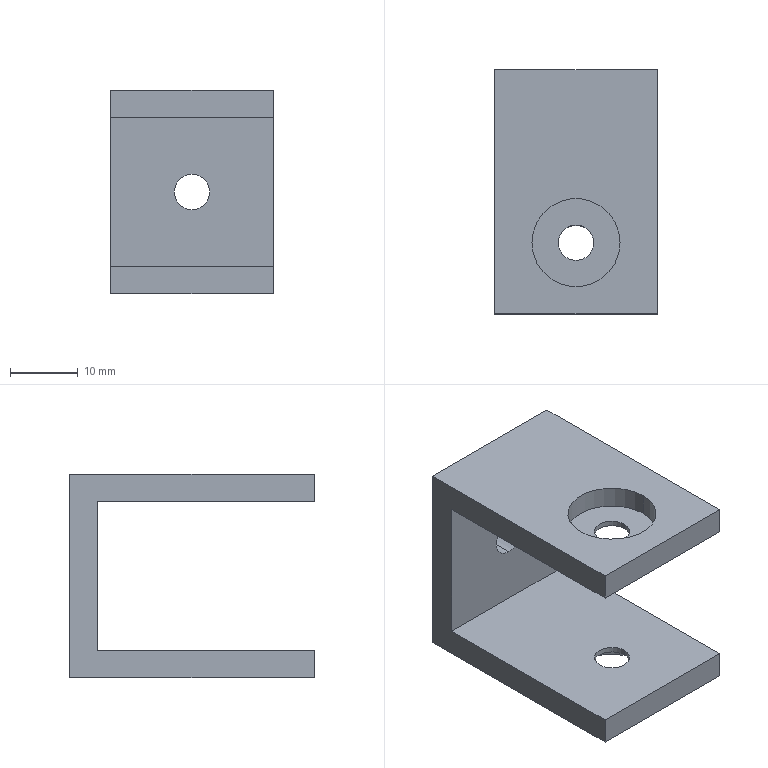Part | SolidWorks | features ICE 12, Extrusion 1, MirrorPattern 1 | 1 solid | 22 faces | box 23.897 x 36 x 30 mm | volume 8017 mm3 | plane 12 | cylinder 10 | commonest cylinder face diameters 5.2 x6 13 x4
STEP:
#1=CARTESIAN_POINT('',(6.5,-14.25,26.8));
#2=VERTEX_POINT('',#1);
#3=CARTESIAN_POINT('',(-6.5,-14.25,26.8));
#4=VERTEX_POINT('',#3);
#5=CARTESIAN_POINT('',(0.,-14.25,26.8));
#6=DIRECTION('',(0.,0.,-1.));
#7=DIRECTION('',(-1.,0.,0.));
#8=AXIS2_PLACEMENT_3D('',#5,#6,#7);
#9=CIRCLE('',#8,6.5);
#10=EDGE_CURVE('',#2,#4,#9,.T.);
#11=ORIENTED_EDGE('',*,*,#10,.T.);
#12=CARTESIAN_POINT('',(-6.5,-14.25,30.));
#13=VERTEX_POINT('',#12);
#14=CARTESIAN_POINT('',(-6.5,-14.25,26.8));
#15=DIRECTION('',(0.,0.,1.));
#16=VECTOR('',#15,1000.);
#17=LINE('',#14,#16);
#18=EDGE_CURVE('',#4,#13,#17,.T.);
#19=ORIENTED_EDGE('',*,*,#18,.T.);
#20=CARTESIAN_POINT('',(6.5,-14.25,30.));
#21=VERTEX_POINT('',#20);
#22=CARTESIAN_POINT('',(0.,-14.25,30.));
#23=DIRECTION('',(0.,0.,-1.));
#24=DIRECTION('',(-1.,0.,0.));
#25=AXIS2_PLACEMENT_3D('',#22,#23,#24);
#26=CIRCLE('',#25,6.5);
#27=EDGE_CURVE('',#21,#13,#26,.T.);
#28=ORIENTED_EDGE('',*,*,#27,.F.);
#29=CARTESIAN_POINT('',(6.5,-14.25,26.8));
#30=DIRECTION('',(0.,0.,1.));
#31=VECTOR('',#30,1000.);
#32=LINE('',#29,#31);
#33=EDGE_CURVE('',#2,#21,#32,.T.);
#34=ORIENTED_EDGE('',*,*,#33,.F.);
#35=EDGE_LOOP('',(#11,#19,#28,#34));
#36=FACE_OUTER_BOUND('',#35,.T.);
#37=CARTESIAN_POINT('',(0.,-14.25,26.8));
#38=DIRECTION('',(0.,0.,1.));
#39=DIRECTION('',(1.,0.,0.));
#40=AXIS2_PLACEMENT_3D('',#37,#38,#39);
#41=CYLINDRICAL_SURFACE('',#40,6.5);
#42=ADVANCED_FACE('',(#36),#41,.F.);
#43=CARTESIAN_POINT('',(6.5,-14.25,3.2));
#44=VERTEX_POINT('',#43);
#45=CARTESIAN_POINT('',(-6.5,-14.25,3.2));
#46=VERTEX_POINT('',#45);
#47=CARTESIAN_POINT('',(0.,-14.25,3.2));
#48=DIRECTION('',(0.,0.,-1.));
#49=DIRECTION('',(-1.,0.,0.));
#50=AXIS2_PLACEMENT_3D('',#47,#48,#49);
#51=CIRCLE('',#50,6.5);
#52=EDGE_CURVE('',#44,#46,#51,.T.);
#53=ORIENTED_EDGE('',*,*,#52,.F.);
#54=CARTESIAN_POINT('',(6.5,-14.25,0.));
#55=VERTEX_POINT('',#54);
#56=CARTESIAN_POINT('',(6.5,-14.25,3.2));
#57=DIRECTION('',(0.,0.,-1.));
#58=VECTOR('',#57,1000.);
#59=LINE('',#56,#58);
#60=EDGE_CURVE('',#44,#55,#59,.T.);
#61=ORIENTED_EDGE('',*,*,#60,.T.);
#62=CARTESIAN_POINT('',(-6.5,-14.25,0.));
#63=VERTEX_POINT('',#62);
#64=CARTESIAN_POINT('',(0.,-14.25,0.));
#65=DIRECTION('',(0.,0.,-1.));
#66=DIRECTION('',(-1.,0.,0.));
#67=AXIS2_PLACEMENT_3D('',#64,#65,#66);
#68=CIRCLE('',#67,6.5);
#69=EDGE_CURVE('',#55,#63,#68,.T.);
#70=ORIENTED_EDGE('',*,*,#69,.T.);
#71=CARTESIAN_POINT('',(-6.5,-14.25,3.2));
#72=DIRECTION('',(0.,0.,-1.));
#73=VECTOR('',#72,1000.);
#74=LINE('',#71,#73);
#75=EDGE_CURVE('',#46,#63,#74,.T.);
#76=ORIENTED_EDGE('',*,*,#75,.F.);
#77=EDGE_LOOP('',(#53,#61,#70,#76));
#78=FACE_OUTER_BOUND('',#77,.T.);
#79=CARTESIAN_POINT('',(0.,-14.25,3.2));
#80=DIRECTION('',(0.,0.,-1.));
#81=DIRECTION('',(-1.,0.,0.));
#82=AXIS2_PLACEMENT_3D('',#79,#80,#81);
#83=CYLINDRICAL_SURFACE('',#82,6.5);
#84=ADVANCED_FACE('',(#78),#83,.F.);
#85=CARTESIAN_POINT('',(0.,7.25,12.4));
#86=VERTEX_POINT('',#85);
#87=CARTESIAN_POINT('',(0.,7.25,17.6));
#88=VERTEX_POINT('',#87);
#89=CARTESIAN_POINT('',(0.,7.25,15.));
#90=DIRECTION('',(0.,1.,0.));
#91=DIRECTION('',(0.,0.,1.));
#92=AXIS2_PLACEMENT_3D('',#89,#90,#91);
#93=CIRCLE('',#92,2.6);
#94=EDGE_CURVE('',#86,#88,#93,.T.);
#95=ORIENTED_EDGE('',*,*,#94,.F.);
#96=CARTESIAN_POINT('',(0.,11.25,12.4));
#97=VERTEX_POINT('',#96);
#98=CARTESIAN_POINT('',(0.,-19.75,12.4));
#99=DIRECTION('',(0.,1.,0.));
#100=VECTOR('',#99,1000.);
#101=LINE('',#98,#100);
#102=EDGE_CURVE('',#86,#97,#101,.T.);
#103=ORIENTED_EDGE('',*,*,#102,.T.);
#104=CARTESIAN_POINT('',(0.,11.25,17.6));
#105=VERTEX_POINT('',#104);
#106=CARTESIAN_POINT('',(0.,11.25,15.));
#107=DIRECTION('',(0.,1.,0.));
#108=DIRECTION('',(0.,0.,1.));
#109=AXIS2_PLACEMENT_3D('',#106,#107,#108);
#110=CIRCLE('',#109,2.6);
#111=EDGE_CURVE('',#97,#105,#110,.T.);
#112=ORIENTED_EDGE('',*,*,#111,.T.);
#113=CARTESIAN_POINT('',(0.,-19.75,17.6));
#114=DIRECTION('',(0.,1.,0.));
#115=VECTOR('',#114,1000.);
#116=LINE('',#113,#115);
#117=EDGE_CURVE('',#88,#105,#116,.T.);
#118=ORIENTED_EDGE('',*,*,#117,.F.);
#119=EDGE_LOOP('',(#95,#103,#112,#118));
#120=FACE_OUTER_BOUND('',#119,.T.);
#121=CARTESIAN_POINT('',(0.,-19.75,15.));
#122=DIRECTION('',(0.,1.,0.));
#123=DIRECTION('',(0.,0.,1.));
#124=AXIS2_PLACEMENT_3D('',#121,#122,#123);
#125=CYLINDRICAL_SURFACE('',#124,2.6);
#126=ADVANCED_FACE('',(#120),#125,.F.);
#127=CARTESIAN_POINT('',(-2.6,-14.25,3.2));
#128=VERTEX_POINT('',#127);
#129=CARTESIAN_POINT('',(2.6,-14.25,3.2));
#130=VERTEX_POINT('',#129);
#131=CARTESIAN_POINT('',(0.,-14.25,3.2));
#132=DIRECTION('',(0.,0.,1.));
#133=DIRECTION('',(-1.,0.,0.));
#134=AXIS2_PLACEMENT_3D('',#131,#132,#133);
#135=CIRCLE('',#134,2.6);
#136=EDGE_CURVE('',#128,#130,#135,.T.);
#137=ORIENTED_EDGE('',*,*,#136,.F.);
#138=CARTESIAN_POINT('',(-2.6,-14.25,4.));
#139=VERTEX_POINT('',#138);
#140=CARTESIAN_POINT('',(-2.6,-14.25,0.));
#141=DIRECTION('',(0.,0.,1.));
#142=VECTOR('',#141,1000.);
#143=LINE('',#140,#142);
#144=EDGE_CURVE('',#128,#139,#143,.T.);
#145=ORIENTED_EDGE('',*,*,#144,.T.);
#146=CARTESIAN_POINT('',(2.6,-14.25,4.));
#147=VERTEX_POINT('',#146);
#148=CARTESIAN_POINT('',(0.,-14.25,4.));
#149=DIRECTION('',(0.,0.,-1.));
#150=DIRECTION('',(0.,1.,0.));
#151=AXIS2_PLACEMENT_3D('',#148,#149,#150);
#152=CIRCLE('',#151,2.6);
#153=EDGE_CURVE('',#147,#139,#152,.T.);
#154=ORIENTED_EDGE('',*,*,#153,.F.);
#155=CARTESIAN_POINT('',(2.6,-14.25,0.));
#156=DIRECTION('',(0.,0.,1.));
#157=VECTOR('',#156,1000.);
#158=LINE('',#155,#157);
#159=EDGE_CURVE('',#130,#147,#158,.T.);
#160=ORIENTED_EDGE('',*,*,#159,.F.);
#161=EDGE_LOOP('',(#137,#145,#154,#160));
#162=FACE_OUTER_BOUND('',#161,.T.);
#163=CARTESIAN_POINT('',(0.,-14.25,0.));
#164=DIRECTION('',(0.,0.,1.));
#165=DIRECTION('',(1.,0.,0.));
#166=AXIS2_PLACEMENT_3D('',#163,#164,#165);
#167=CYLINDRICAL_SURFACE('',#166,2.6);
#168=ADVANCED_FACE('',(#162),#167,.F.);
#169=CARTESIAN_POINT('',(-2.6,-14.25,26.));
#170=VERTEX_POINT('',#169);
#171=CARTESIAN_POINT('',(2.6,-14.25,26.));
#172=VERTEX_POINT('',#171);
#173=CARTESIAN_POINT('',(0.,-14.25,26.));
#174=DIRECTION('',(0.,0.,1.));
#175=DIRECTION('',(0.,-1.,0.));
#176=AXIS2_PLACEMENT_3D('',#173,#174,#175);
#177=CIRCLE('',#176,2.6);
#178=EDGE_CURVE('',#170,#172,#177,.T.);
#179=ORIENTED_EDGE('',*,*,#178,.F.);
#180=CARTESIAN_POINT('',(-2.6,-14.25,26.8));
#181=VERTEX_POINT('',#180);
#182=CARTESIAN_POINT('',(-2.6,-14.25,0.));
#183=DIRECTION('',(0.,0.,1.));
#184=VECTOR('',#183,1000.);
#185=LINE('',#182,#184);
#186=EDGE_CURVE('',#170,#181,#185,.T.);
#187=ORIENTED_EDGE('',*,*,#186,.T.);
#188=CARTESIAN_POINT('',(2.6,-14.25,26.8));
#189=VERTEX_POINT('',#188);
#190=CARTESIAN_POINT('',(0.,-14.25,26.8));
#191=DIRECTION('',(0.,0.,-1.));
#192=DIRECTION('',(1.,0.,0.));
#193=AXIS2_PLACEMENT_3D('',#190,#191,#192);
#194=CIRCLE('',#193,2.6);
#195=EDGE_CURVE('',#189,#181,#194,.T.);
#196=ORIENTED_EDGE('',*,*,#195,.F.);
#197=CARTESIAN_POINT('',(2.6,-14.25,0.));
#198=DIRECTION('',(0.,0.,1.));
#199=VECTOR('',#198,1000.);
#200=LINE('',#197,#199);
#201=EDGE_CURVE('',#172,#189,#200,.T.);
#202=ORIENTED_EDGE('',*,*,#201,.F.);
#203=EDGE_LOOP('',(#179,#187,#196,#202));
#204=FACE_OUTER_BOUND('',#203,.T.);
#205=CARTESIAN_POINT('',(0.,-14.25,0.));
#206=DIRECTION('',(0.,0.,1.));
#207=DIRECTION('',(1.,0.,0.));
#208=AXIS2_PLACEMENT_3D('',#205,#206,#207);
#209=CYLINDRICAL_SURFACE('',#208,2.6);
#210=ADVANCED_FACE('',(#204),#209,.F.);
#211=ORIENTED_EDGE('',*,*,#186,.F.);
#212=CARTESIAN_POINT('',(0.,-14.25,26.));
#213=DIRECTION('',(0.,0.,1.));
#214=DIRECTION('',(0.,-1.,0.));
#215=AXIS2_PLACEMENT_3D('',#212,#213,#214);
#216=CIRCLE('',#215,2.6);
#217=EDGE_CURVE('',#172,#170,#216,.T.);
#218=ORIENTED_EDGE('',*,*,#217,.F.);
#219=ORIENTED_EDGE('',*,*,#201,.T.);
#220=CARTESIAN_POINT('',(0.,-14.25,26.8));
#221=DIRECTION('',(0.,0.,-1.));
#222=DIRECTION('',(1.,0.,0.));
#223=AXIS2_PLACEMENT_3D('',#220,#221,#222);
#224=CIRCLE('',#223,2.6);
#225=EDGE_CURVE('',#181,#189,#224,.T.);
#226=ORIENTED_EDGE('',*,*,#225,.F.);
#227=EDGE_LOOP('',(#211,#218,#219,#226));
#228=FACE_OUTER_BOUND('',#227,.T.);
#229=CARTESIAN_POINT('',(0.,-14.25,0.));
#230=DIRECTION('',(0.,0.,1.));
#231=DIRECTION('',(1.,0.,0.));
#232=AXIS2_PLACEMENT_3D('',#229,#230,#231);
#233=CYLINDRICAL_SURFACE('',#232,2.6);
#234=ADVANCED_FACE('',(#228),#233,.F.);
#235=ORIENTED_EDGE('',*,*,#144,.F.);
#236=CARTESIAN_POINT('',(0.,-14.25,3.2));
#237=DIRECTION('',(0.,0.,1.));
#238=DIRECTION('',(-1.,0.,0.));
#239=AXIS2_PLACEMENT_3D('',#236,#237,#238);
#240=CIRCLE('',#239,2.6);
#241=EDGE_CURVE('',#130,#128,#240,.T.);
#242=ORIENTED_EDGE('',*,*,#241,.F.);
#243=ORIENTED_EDGE('',*,*,#159,.T.);
#244=CARTESIAN_POINT('',(0.,-14.25,4.));
#245=DIRECTION('',(0.,0.,-1.));
#246=DIRECTION('',(0.,1.,0.));
#247=AXIS2_PLACEMENT_3D('',#244,#245,#246);
#248=CIRCLE('',#247,2.6);
#249=EDGE_CURVE('',#139,#147,#248,.T.);
#250=ORIENTED_EDGE('',*,*,#249,.F.);
#251=EDGE_LOOP('',(#235,#242,#243,#250));
#252=FACE_OUTER_BOUND('',#251,.T.);
#253=CARTESIAN_POINT('',(0.,-14.25,0.));
#254=DIRECTION('',(0.,0.,1.));
#255=DIRECTION('',(1.,0.,0.));
#256=AXIS2_PLACEMENT_3D('',#253,#254,#255);
#257=CYLINDRICAL_SURFACE('',#256,2.6);
#258=ADVANCED_FACE('',(#252),#257,.F.);
#259=CARTESIAN_POINT('',(11.948,-24.75,0.));
#260=VERTEX_POINT('',#259);
#261=CARTESIAN_POINT('',(11.948,11.25,0.));
#262=VERTEX_POINT('',#261);
#263=CARTESIAN_POINT('',(11.948,12.75,0.));
#264=DIRECTION('',(0.,1.,0.));
#265=VECTOR('',#264,1000.);
#266=LINE('',#263,#265);
#267=EDGE_CURVE('',#260,#262,#266,.T.);
#268=ORIENTED_EDGE('',*,*,#267,.T.);
#269=CARTESIAN_POINT('',(11.948,11.25,30.));
#270=VERTEX_POINT('',#269);
#271=CARTESIAN_POINT('',(11.948,11.25,30.));
#272=DIRECTION('',(0.,0.,-1.));
#273=VECTOR('',#272,1000.);
#274=LINE('',#271,#273);
#275=EDGE_CURVE('',#270,#262,#274,.T.);
#276=ORIENTED_EDGE('',*,*,#275,.F.);
#277=CARTESIAN_POINT('',(11.948,-24.75,30.));
#278=VERTEX_POINT('',#277);
#279=CARTESIAN_POINT('',(11.948,12.75,30.));
#280=DIRECTION('',(0.,1.,0.));
#281=VECTOR('',#280,1000.);
#282=LINE('',#279,#281);
#283=EDGE_CURVE('',#278,#270,#282,.T.);
#284=ORIENTED_EDGE('',*,*,#283,.F.);
#285=CARTESIAN_POINT('',(11.948,-24.75,26.));
#286=VERTEX_POINT('',#285);
#287=CARTESIAN_POINT('',(11.948,-24.75,26.));
#288=DIRECTION('',(0.,0.,1.));
#289=VECTOR('',#288,1000.);
#290=LINE('',#287,#289);
#291=EDGE_CURVE('',#286,#278,#290,.T.);
#292=ORIENTED_EDGE('',*,*,#291,.F.);
#293=CARTESIAN_POINT('',(11.948,7.25,26.));
#294=VERTEX_POINT('',#293);
#295=CARTESIAN_POINT('',(11.948,7.25,26.));
#296=DIRECTION('',(0.,-1.,0.));
#297=VECTOR('',#296,1000.);
#298=LINE('',#295,#297);
#299=EDGE_CURVE('',#294,#286,#298,.T.);
#300=ORIENTED_EDGE('',*,*,#299,.F.);
#301=CARTESIAN_POINT('',(11.948,7.25,4.));
#302=VERTEX_POINT('',#301);
#303=CARTESIAN_POINT('',(11.948,7.25,20.));
#304=DIRECTION('',(0.,0.,1.));
#305=VECTOR('',#304,1000.);
#306=LINE('',#303,#305);
#307=EDGE_CURVE('',#302,#294,#306,.T.);
#308=ORIENTED_EDGE('',*,*,#307,.F.);
#309=CARTESIAN_POINT('',(11.948,-24.75,4.));
#310=VERTEX_POINT('',#309);
#311=CARTESIAN_POINT('',(11.948,7.25,4.));
#312=DIRECTION('',(0.,1.,0.));
#313=VECTOR('',#312,1000.);
#314=LINE('',#311,#313);
#315=EDGE_CURVE('',#310,#302,#314,.T.);
#316=ORIENTED_EDGE('',*,*,#315,.F.);
#317=CARTESIAN_POINT('',(11.948,-24.75,0.));
#318=DIRECTION('',(0.,0.,1.));
#319=VECTOR('',#318,1000.);
#320=LINE('',#317,#319);
#321=EDGE_CURVE('',#260,#310,#320,.T.);
#322=ORIENTED_EDGE('',*,*,#321,.F.);
#323=EDGE_LOOP('',(#268,#276,#284,#292,#300,#308,#316,#322));
#324=FACE_OUTER_BOUND('',#323,.T.);
#325=CARTESIAN_POINT('',(11.948,12.75,30.));
#326=DIRECTION('',(-1.,0.,0.));
#327=DIRECTION('',(0.,0.,1.));
#328=AXIS2_PLACEMENT_3D('',#325,#326,#327);
#329=PLANE('',#328);
#330=ADVANCED_FACE('',(#324),#329,.F.);
#331=CARTESIAN_POINT('',(-11.948,11.25,30.));
#332=VERTEX_POINT('',#331);
#333=CARTESIAN_POINT('',(-11.948,-24.75,30.));
#334=VERTEX_POINT('',#333);
#335=CARTESIAN_POINT('',(-11.948,12.75,30.));
#336=DIRECTION('',(0.,-1.,0.));
#337=VECTOR('',#336,1000.);
#338=LINE('',#335,#337);
#339=EDGE_CURVE('',#332,#334,#338,.T.);
#340=ORIENTED_EDGE('',*,*,#339,.F.);
#341=CARTESIAN_POINT('',(-11.948,11.25,0.));
#342=VERTEX_POINT('',#341);
#343=CARTESIAN_POINT('',(-11.948,11.25,30.));
#344=DIRECTION('',(0.,0.,-1.));
#345=VECTOR('',#344,1000.);
#346=LINE('',#343,#345);
#347=EDGE_CURVE('',#332,#342,#346,.T.);
#348=ORIENTED_EDGE('',*,*,#347,.T.);
#349=CARTESIAN_POINT('',(-11.948,-24.75,0.));
#350=VERTEX_POINT('',#349);
#351=CARTESIAN_POINT('',(-11.948,12.75,0.));
#352=DIRECTION('',(0.,-1.,0.));
#353=VECTOR('',#352,1000.);
#354=LINE('',#351,#353);
#355=EDGE_CURVE('',#342,#350,#354,.T.);
#356=ORIENTED_EDGE('',*,*,#355,.T.);
#357=CARTESIAN_POINT('',(-11.948,-24.75,4.));
#358=VERTEX_POINT('',#357);
#359=CARTESIAN_POINT('',(-11.948,-24.75,4.));
#360=DIRECTION('',(0.,0.,-1.));
#361=VECTOR('',#360,1000.);
#362=LINE('',#359,#361);
#363=EDGE_CURVE('',#358,#350,#362,.T.);
#364=ORIENTED_EDGE('',*,*,#363,.F.);
#365=CARTESIAN_POINT('',(-11.948,7.25,4.));
#366=VERTEX_POINT('',#365);
#367=CARTESIAN_POINT('',(-11.948,7.25,4.));
#368=DIRECTION('',(0.,-1.,0.));
#369=VECTOR('',#368,1000.);
#370=LINE('',#367,#369);
#371=EDGE_CURVE('',#366,#358,#370,.T.);
#372=ORIENTED_EDGE('',*,*,#371,.F.);
#373=CARTESIAN_POINT('',(-11.948,7.25,26.));
#374=VERTEX_POINT('',#373);
#375=CARTESIAN_POINT('',(-11.948,7.25,20.));
#376=DIRECTION('',(0.,0.,1.));
#377=VECTOR('',#376,1000.);
#378=LINE('',#375,#377);
#379=EDGE_CURVE('',#366,#374,#378,.T.);
#380=ORIENTED_EDGE('',*,*,#379,.T.);
#381=CARTESIAN_POINT('',(-11.948,-24.75,26.));
#382=VERTEX_POINT('',#381);
#383=CARTESIAN_POINT('',(-11.948,7.25,26.));
#384=DIRECTION('',(0.,1.,0.));
#385=VECTOR('',#384,1000.);
#386=LINE('',#383,#385);
#387=EDGE_CURVE('',#382,#374,#386,.T.);
#388=ORIENTED_EDGE('',*,*,#387,.F.);
#389=CARTESIAN_POINT('',(-11.948,-24.75,30.));
#390=DIRECTION('',(0.,0.,-1.));
#391=VECTOR('',#390,1000.);
#392=LINE('',#389,#391);
#393=EDGE_CURVE('',#334,#382,#392,.T.);
#394=ORIENTED_EDGE('',*,*,#393,.F.);
#395=EDGE_LOOP('',(#340,#348,#356,#364,#372,#380,#388,#394));
#396=FACE_OUTER_BOUND('',#395,.T.);
#397=CARTESIAN_POINT('',(-11.948,12.75,30.));
#398=DIRECTION('',(1.,0.,0.));
#399=DIRECTION('',(0.,0.,-1.));
#400=AXIS2_PLACEMENT_3D('',#397,#398,#399);
#401=PLANE('',#400);
#402=ADVANCED_FACE('',(#396),#401,.F.);
#403=ORIENTED_EDGE('',*,*,#27,.T.);
#404=CARTESIAN_POINT('',(0.,-14.25,30.));
#405=DIRECTION('',(0.,0.,-1.));
#406=DIRECTION('',(-1.,0.,0.));
#407=AXIS2_PLACEMENT_3D('',#404,#405,#406);
#408=CIRCLE('',#407,6.5);
#409=EDGE_CURVE('',#13,#21,#408,.T.);
#410=ORIENTED_EDGE('',*,*,#409,.T.);
#411=EDGE_LOOP('',(#403,#410));
#412=FACE_BOUND('',#411,.T.);
#413=CARTESIAN_POINT('',(-11.948,11.25,30.));
#414=DIRECTION('',(1.,0.,0.));
#415=VECTOR('',#414,1000.);
#416=LINE('',#413,#415);
#417=EDGE_CURVE('',#332,#270,#416,.T.);
#418=ORIENTED_EDGE('',*,*,#417,.F.);
#419=ORIENTED_EDGE('',*,*,#339,.T.);
#420=CARTESIAN_POINT('',(11.948,-24.75,30.));
#421=DIRECTION('',(-1.,0.,0.));
#422=VECTOR('',#421,1000.);
#423=LINE('',#420,#422);
#424=EDGE_CURVE('',#278,#334,#423,.T.);
#425=ORIENTED_EDGE('',*,*,#424,.F.);
#426=ORIENTED_EDGE('',*,*,#283,.T.);
#427=EDGE_LOOP('',(#418,#419,#425,#426));
#428=FACE_OUTER_BOUND('',#427,.T.);
#429=CARTESIAN_POINT('',(0.,0.,30.));
#430=DIRECTION('',(0.,0.,1.));
#431=DIRECTION('',(1.,0.,0.));
#432=AXIS2_PLACEMENT_3D('',#429,#430,#431);
#433=PLANE('',#432);
#434=ADVANCED_FACE('',(#412,#428),#433,.T.);
#435=CARTESIAN_POINT('',(0.,-14.25,0.));
#436=DIRECTION('',(0.,0.,-1.));
#437=DIRECTION('',(-1.,0.,0.));
#438=AXIS2_PLACEMENT_3D('',#435,#436,#437);
#439=CIRCLE('',#438,6.5);
#440=EDGE_CURVE('',#63,#55,#439,.T.);
#441=ORIENTED_EDGE('',*,*,#440,.F.);
#442=ORIENTED_EDGE('',*,*,#69,.F.);
#443=EDGE_LOOP('',(#441,#442));
#444=FACE_BOUND('',#443,.T.);
#445=ORIENTED_EDGE('',*,*,#355,.F.);
#446=CARTESIAN_POINT('',(-11.948,11.25,0.));
#447=DIRECTION('',(1.,0.,0.));
#448=VECTOR('',#447,1000.);
#449=LINE('',#446,#448);
#450=EDGE_CURVE('',#342,#262,#449,.T.);
#451=ORIENTED_EDGE('',*,*,#450,.T.);
#452=ORIENTED_EDGE('',*,*,#267,.F.);
#453=CARTESIAN_POINT('',(-11.948,-24.75,0.));
#454=DIRECTION('',(1.,0.,0.));
#455=VECTOR('',#454,1000.);
#456=LINE('',#453,#455);
#457=EDGE_CURVE('',#350,#260,#456,.T.);
#458=ORIENTED_EDGE('',*,*,#457,.F.);
#459=EDGE_LOOP('',(#445,#451,#452,#458));
#460=FACE_OUTER_BOUND('',#459,.T.);
#461=CARTESIAN_POINT('',(0.,0.,0.));
#462=DIRECTION('',(0.,0.,1.));
#463=DIRECTION('',(1.,0.,0.));
#464=AXIS2_PLACEMENT_3D('',#461,#462,#463);
#465=PLANE('',#464);
#466=ADVANCED_FACE('',(#444,#460),#465,.F.);
#467=CARTESIAN_POINT('',(0.,7.25,15.));
#468=DIRECTION('',(0.,1.,0.));
#469=DIRECTION('',(0.,0.,1.));
#470=AXIS2_PLACEMENT_3D('',#467,#468,#469);
#471=CIRCLE('',#470,2.6);
#472=EDGE_CURVE('',#88,#86,#471,.T.);
#473=ORIENTED_EDGE('',*,*,#472,.T.);
#474=ORIENTED_EDGE('',*,*,#94,.T.);
#475=EDGE_LOOP('',(#473,#474));
#476=FACE_BOUND('',#475,.T.);
#477=ORIENTED_EDGE('',*,*,#307,.T.);
#478=CARTESIAN_POINT('',(32.829,7.25,26.));
#479=DIRECTION('',(-1.,0.,0.));
#480=VECTOR('',#479,1000.);
#481=LINE('',#478,#480);
#482=EDGE_CURVE('',#294,#374,#481,.T.);
#483=ORIENTED_EDGE('',*,*,#482,.T.);
#484=ORIENTED_EDGE('',*,*,#379,.F.);
#485=CARTESIAN_POINT('',(32.829,7.25,4.));
#486=DIRECTION('',(-1.,0.,0.));
#487=VECTOR('',#486,1000.);
#488=LINE('',#485,#487);
#489=EDGE_CURVE('',#302,#366,#488,.T.);
#490=ORIENTED_EDGE('',*,*,#489,.F.);
#491=EDGE_LOOP('',(#477,#483,#484,#490));
#492=FACE_OUTER_BOUND('',#491,.T.);
#493=CARTESIAN_POINT('',(-11.948,7.25,20.));
#494=DIRECTION('',(0.,1.,0.));
#495=DIRECTION('',(0.,0.,1.));
#496=AXIS2_PLACEMENT_3D('',#493,#494,#495);
#497=PLANE('',#496);
#498=ADVANCED_FACE('',(#476,#492),#497,.F.);
#499=ORIENTED_EDGE('',*,*,#217,.T.);
#500=ORIENTED_EDGE('',*,*,#178,.T.);
#501=EDGE_LOOP('',(#499,#500));
#502=FACE_BOUND('',#501,.T.);
#503=ORIENTED_EDGE('',*,*,#299,.T.);
#504=CARTESIAN_POINT('',(-11.948,-24.75,26.));
#505=DIRECTION('',(1.,0.,0.));
#506=VECTOR('',#505,1000.);
#507=LINE('',#504,#506);
#508=EDGE_CURVE('',#382,#286,#507,.T.);
#509=ORIENTED_EDGE('',*,*,#508,.F.);
#510=ORIENTED_EDGE('',*,*,#387,.T.);
#511=ORIENTED_EDGE('',*,*,#482,.F.);
#512=EDGE_LOOP('',(#503,#509,#510,#511));
#513=FACE_OUTER_BOUND('',#512,.T.);
#514=CARTESIAN_POINT('',(32.829,7.25,26.));
#515=DIRECTION('',(0.,0.,1.));
#516=DIRECTION('',(0.,-1.,0.));
#517=AXIS2_PLACEMENT_3D('',#514,#515,#516);
#518=PLANE('',#517);
#519=ADVANCED_FACE('',(#502,#513),#518,.F.);
#520=ORIENTED_EDGE('',*,*,#153,.T.);
#521=ORIENTED_EDGE('',*,*,#249,.T.);
#522=EDGE_LOOP('',(#520,#521));
#523=FACE_BOUND('',#522,.T.);
#524=ORIENTED_EDGE('',*,*,#315,.T.);
#525=ORIENTED_EDGE('',*,*,#489,.T.);
#526=ORIENTED_EDGE('',*,*,#371,.T.);
#527=CARTESIAN_POINT('',(11.948,-24.75,4.));
#528=DIRECTION('',(-1.,0.,0.));
#529=VECTOR('',#528,1000.);
#530=LINE('',#527,#529);
#531=EDGE_CURVE('',#310,#358,#530,.T.);
#532=ORIENTED_EDGE('',*,*,#531,.F.);
#533=EDGE_LOOP('',(#524,#525,#526,#532));
#534=FACE_OUTER_BOUND('',#533,.T.);
#535=CARTESIAN_POINT('',(32.829,7.25,4.));
#536=DIRECTION('',(0.,0.,-1.));
#537=DIRECTION('',(0.,1.,0.));
#538=AXIS2_PLACEMENT_3D('',#535,#536,#537);
#539=PLANE('',#538);
#540=ADVANCED_FACE('',(#523,#534),#539,.F.);
#541=CARTESIAN_POINT('',(0.,11.25,15.));
#542=DIRECTION('',(0.,1.,0.));
#543=DIRECTION('',(0.,0.,1.));
#544=AXIS2_PLACEMENT_3D('',#541,#542,#543);
#545=CIRCLE('',#544,2.6);
#546=EDGE_CURVE('',#105,#97,#545,.T.);
#547=ORIENTED_EDGE('',*,*,#546,.F.);
#548=ORIENTED_EDGE('',*,*,#111,.F.);
#549=EDGE_LOOP('',(#547,#548));
#550=FACE_BOUND('',#549,.T.);
#551=ORIENTED_EDGE('',*,*,#275,.T.);
#552=ORIENTED_EDGE('',*,*,#450,.F.);
#553=ORIENTED_EDGE('',*,*,#347,.F.);
#554=ORIENTED_EDGE('',*,*,#417,.T.);
#555=EDGE_LOOP('',(#551,#552,#553,#554));
#556=FACE_OUTER_BOUND('',#555,.T.);
#557=CARTESIAN_POINT('',(-11.948,11.25,30.));
#558=DIRECTION('',(0.,-1.,0.));
#559=DIRECTION('',(0.,0.,-1.));
#560=AXIS2_PLACEMENT_3D('',#557,#558,#559);
#561=PLANE('',#560);
#562=ADVANCED_FACE('',(#550,#556),#561,.F.);
#563=ORIENTED_EDGE('',*,*,#102,.F.);
#564=ORIENTED_EDGE('',*,*,#472,.F.);
#565=ORIENTED_EDGE('',*,*,#117,.T.);
#566=ORIENTED_EDGE('',*,*,#546,.T.);
#567=EDGE_LOOP('',(#563,#564,#565,#566));
#568=FACE_OUTER_BOUND('',#567,.T.);
#569=CARTESIAN_POINT('',(0.,-19.75,15.));
#570=DIRECTION('',(0.,1.,0.));
#571=DIRECTION('',(0.,0.,1.));
#572=AXIS2_PLACEMENT_3D('',#569,#570,#571);
#573=CYLINDRICAL_SURFACE('',#572,2.6);
#574=ADVANCED_FACE('',(#568),#573,.F.);
#575=ORIENTED_EDGE('',*,*,#363,.T.);
#576=ORIENTED_EDGE('',*,*,#457,.T.);
#577=ORIENTED_EDGE('',*,*,#321,.T.);
#578=ORIENTED_EDGE('',*,*,#531,.T.);
#579=EDGE_LOOP('',(#575,#576,#577,#578));
#580=FACE_OUTER_BOUND('',#579,.T.);
#581=CARTESIAN_POINT('',(0.,-24.75,0.));
#582=DIRECTION('',(0.,-1.,0.));
#583=DIRECTION('',(0.,0.,-1.));
#584=AXIS2_PLACEMENT_3D('',#581,#582,#583);
#585=PLANE('',#584);
#586=ADVANCED_FACE('',(#580),#585,.T.);
#587=ORIENTED_EDGE('',*,*,#291,.T.);
#588=ORIENTED_EDGE('',*,*,#424,.T.);
#589=ORIENTED_EDGE('',*,*,#393,.T.);
#590=ORIENTED_EDGE('',*,*,#508,.T.);
#591=EDGE_LOOP('',(#587,#588,#589,#590));
#592=FACE_OUTER_BOUND('',#591,.T.);
#593=CARTESIAN_POINT('',(0.,-24.75,0.));
#594=DIRECTION('',(0.,-1.,0.));
#595=DIRECTION('',(0.,0.,-1.));
#596=AXIS2_PLACEMENT_3D('',#593,#594,#595);
#597=PLANE('',#596);
#598=ADVANCED_FACE('',(#592),#597,.T.);
#599=CARTESIAN_POINT('',(0.,-14.25,3.2));
#600=DIRECTION('',(0.,0.,-1.));
#601=DIRECTION('',(-1.,0.,0.));
#602=AXIS2_PLACEMENT_3D('',#599,#600,#601);
#603=CIRCLE('',#602,6.5);
#604=EDGE_CURVE('',#46,#44,#603,.T.);
#605=ORIENTED_EDGE('',*,*,#604,.T.);
#606=ORIENTED_EDGE('',*,*,#52,.T.);
#607=EDGE_LOOP('',(#605,#606));
#608=FACE_OUTER_BOUND('',#607,.T.);
#609=ORIENTED_EDGE('',*,*,#241,.T.);
#610=ORIENTED_EDGE('',*,*,#136,.T.);
#611=EDGE_LOOP('',(#609,#610));
#612=FACE_BOUND('',#611,.T.);
#613=CARTESIAN_POINT('',(0.,-14.25,3.2));
#614=DIRECTION('',(0.,0.,-1.));
#615=DIRECTION('',(-1.,0.,0.));
#616=AXIS2_PLACEMENT_3D('',#613,#614,#615);
#617=PLANE('',#616);
#618=ADVANCED_FACE('',(#608,#612),#617,.T.);
#619=ORIENTED_EDGE('',*,*,#60,.F.);
#620=ORIENTED_EDGE('',*,*,#604,.F.);
#621=ORIENTED_EDGE('',*,*,#75,.T.);
#622=ORIENTED_EDGE('',*,*,#440,.T.);
#623=EDGE_LOOP('',(#619,#620,#621,#622));
#624=FACE_OUTER_BOUND('',#623,.T.);
#625=CARTESIAN_POINT('',(0.,-14.25,3.2));
#626=DIRECTION('',(0.,0.,-1.));
#627=DIRECTION('',(-1.,0.,0.));
#628=AXIS2_PLACEMENT_3D('',#625,#626,#627);
#629=CYLINDRICAL_SURFACE('',#628,6.5);
#630=ADVANCED_FACE('',(#624),#629,.F.);
#631=ORIENTED_EDGE('',*,*,#10,.F.);
#632=CARTESIAN_POINT('',(0.,-14.25,26.8));
#633=DIRECTION('',(0.,0.,-1.));
#634=DIRECTION('',(-1.,0.,0.));
#635=AXIS2_PLACEMENT_3D('',#632,#633,#634);
#636=CIRCLE('',#635,6.5);
#637=EDGE_CURVE('',#4,#2,#636,.T.);
#638=ORIENTED_EDGE('',*,*,#637,.F.);
#639=EDGE_LOOP('',(#631,#638));
#640=FACE_OUTER_BOUND('',#639,.T.);
#641=ORIENTED_EDGE('',*,*,#195,.T.);
#642=ORIENTED_EDGE('',*,*,#225,.T.);
#643=EDGE_LOOP('',(#641,#642));
#644=FACE_BOUND('',#643,.T.);
#645=CARTESIAN_POINT('',(0.,-14.25,26.8));
#646=DIRECTION('',(0.,0.,1.));
#647=DIRECTION('',(-1.,0.,0.));
#648=AXIS2_PLACEMENT_3D('',#645,#646,#647);
#649=PLANE('',#648);
#650=ADVANCED_FACE('',(#640,#644),#649,.T.);
#651=ORIENTED_EDGE('',*,*,#18,.F.);
#652=ORIENTED_EDGE('',*,*,#637,.T.);
#653=ORIENTED_EDGE('',*,*,#33,.T.);
#654=ORIENTED_EDGE('',*,*,#409,.F.);
#655=EDGE_LOOP('',(#651,#652,#653,#654));
#656=FACE_OUTER_BOUND('',#655,.T.);
#657=CARTESIAN_POINT('',(0.,-14.25,26.8));
#658=DIRECTION('',(0.,0.,1.));
#659=DIRECTION('',(1.,0.,0.));
#660=AXIS2_PLACEMENT_3D('',#657,#658,#659);
#661=CYLINDRICAL_SURFACE('',#660,6.5);
#662=ADVANCED_FACE('',(#656),#661,.F.);
#663=CLOSED_SHELL('',(#42,#84,#126,#168,#210,#234,#258,#330,#402,#434,#466,#498,#519,#540,#562,#574,#586,#598,#618,#630,#650,#662));
#664=MANIFOLD_SOLID_BREP('',#663);
#665=CARTESIAN_POINT('',(0.,0.,0.));
#666=DIRECTION('',(0.,0.,1.));
#667=DIRECTION('',(1.,0.,0.));
#668=AXIS2_PLACEMENT_3D('',#665,#666,#667);
#669=(LENGTH_UNIT()NAMED_UNIT(*)SI_UNIT(.MILLI.,.METRE.));
#670=UNCERTAINTY_MEASURE_WITH_UNIT(LENGTH_MEASURE(0.00001),#669,'','');
#671=(NAMED_UNIT(*)PLANE_ANGLE_UNIT()SI_UNIT($,.RADIAN.));
#672=(NAMED_UNIT(*)SI_UNIT($,.STERADIAN.)SOLID_ANGLE_UNIT());
#673=(GEOMETRIC_REPRESENTATION_CONTEXT(3)GLOBAL_UNCERTAINTY_ASSIGNED_CONTEXT((#670))GLOBAL_UNIT_ASSIGNED_CONTEXT((#669,#671,#672))REPRESENTATION_CONTEXT('',''));
#674=ADVANCED_BREP_SHAPE_REPRESENTATION('',(#664,#668),#673);